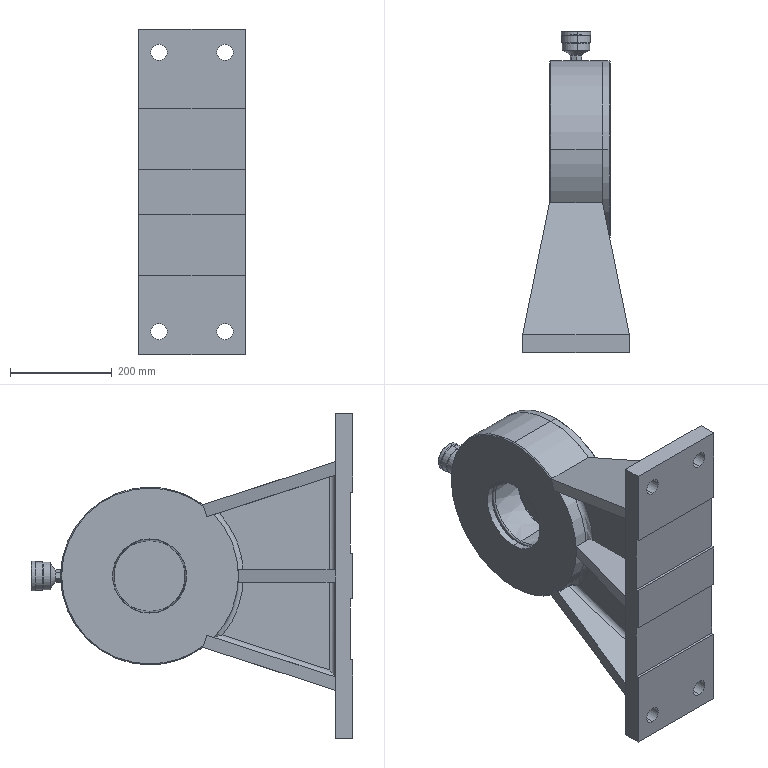Part | SolidWorks | 5 solids | 361 faces | box 210 x 633 x 640 mm | volume 18025314 mm3 | plane 132 | torus 88 | cylinder 72 | cone 67 | sphere 2 | commonest cylinder face diameters 14 x12 18 x12 32 x8 350 x7 250 x6 20 x5